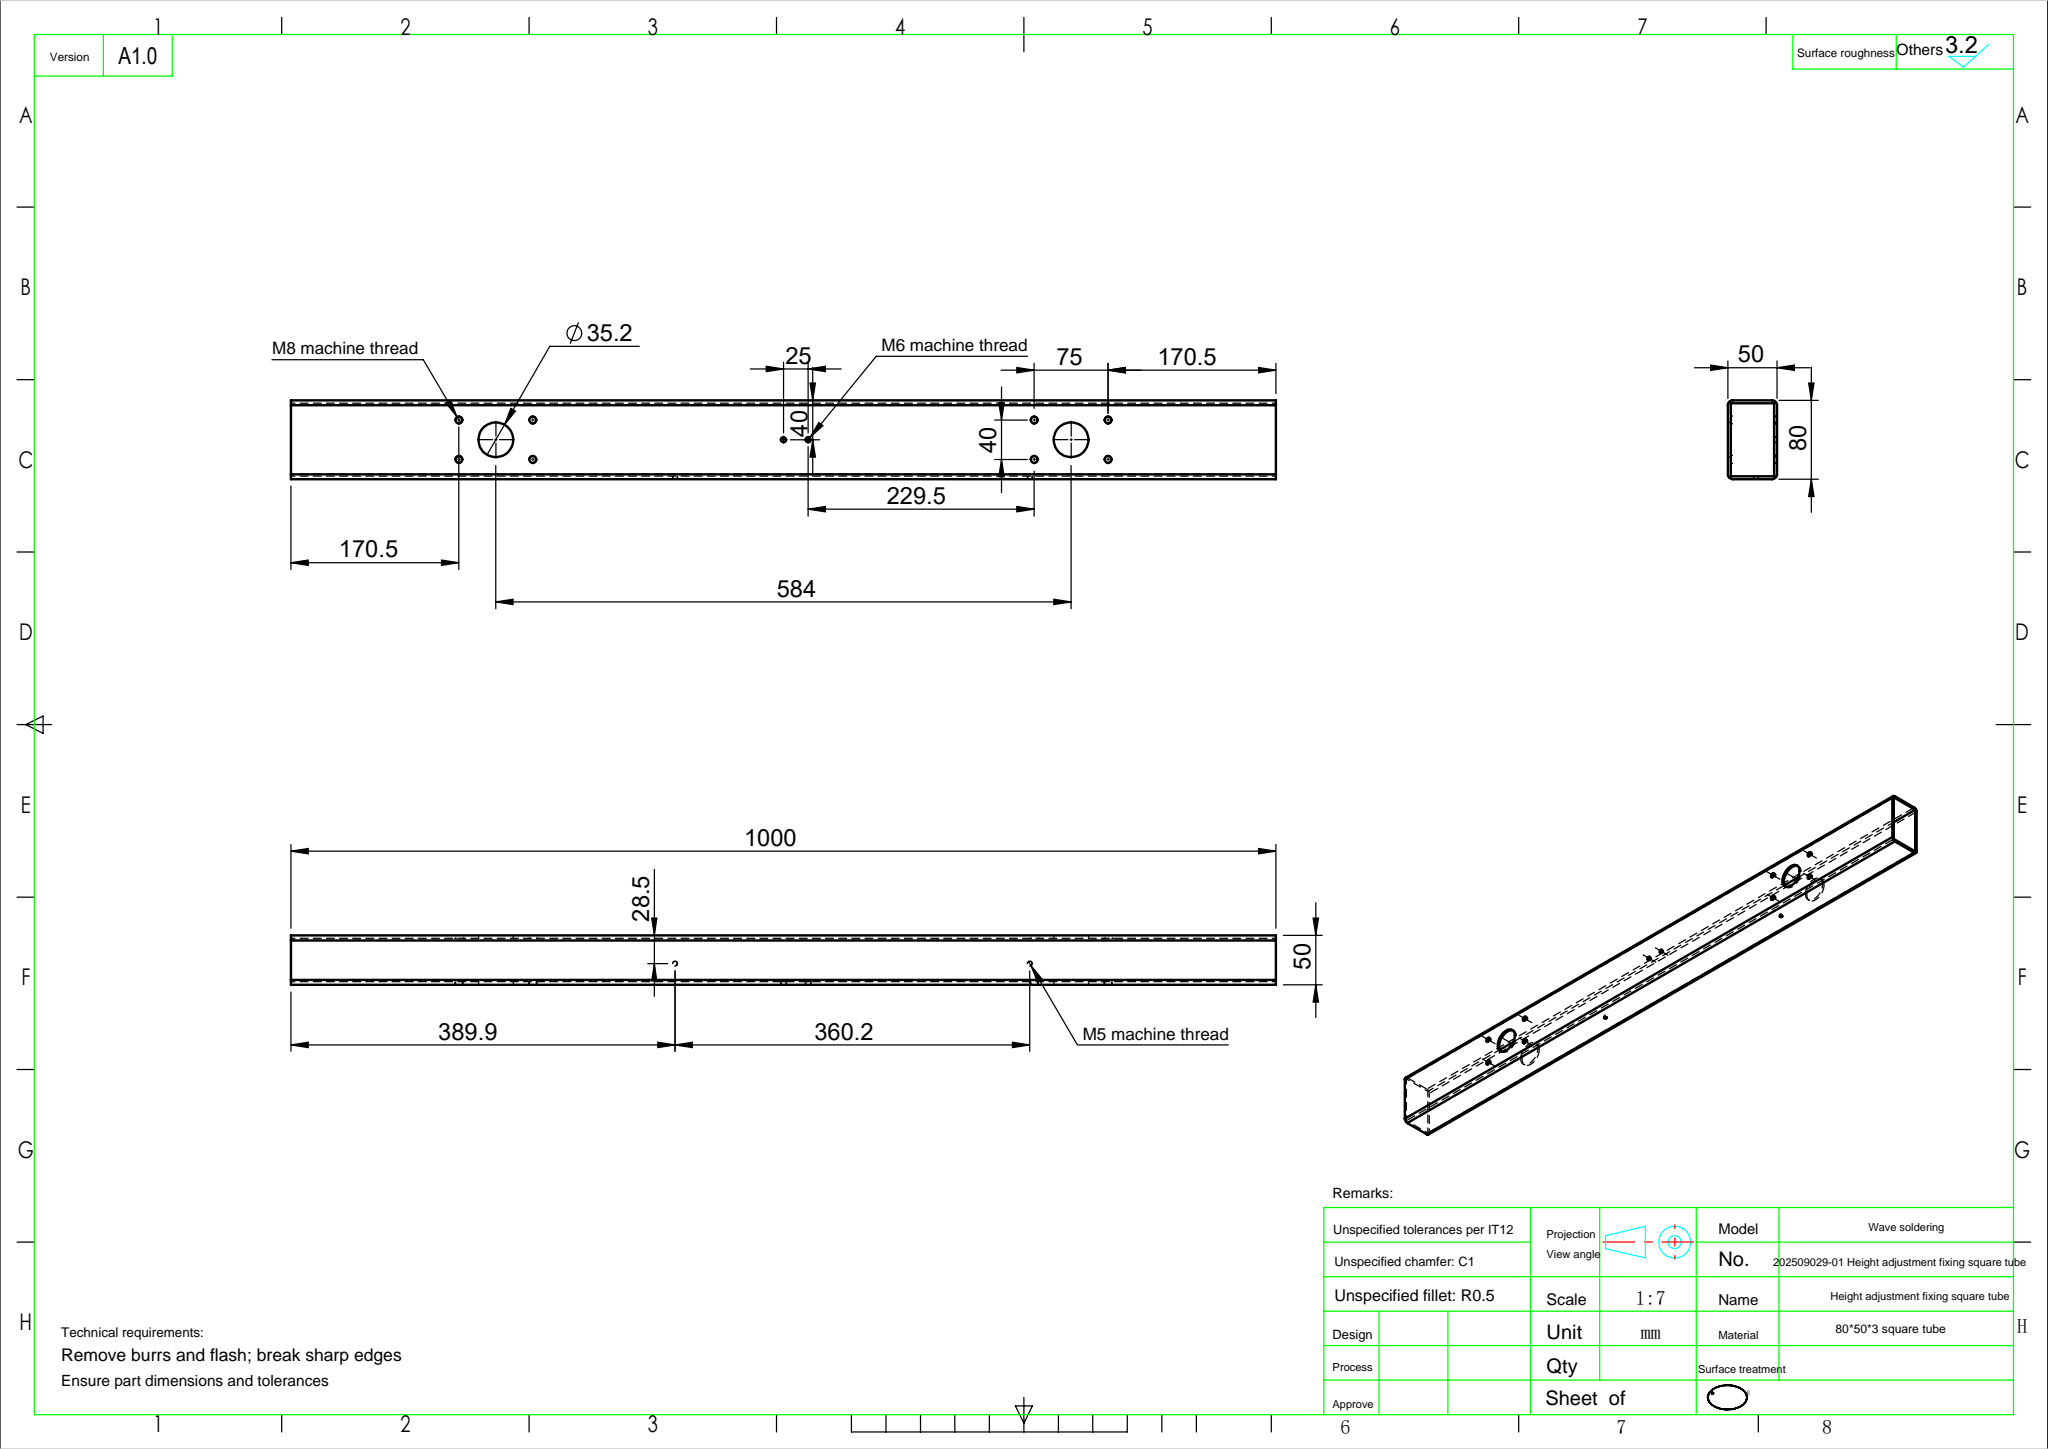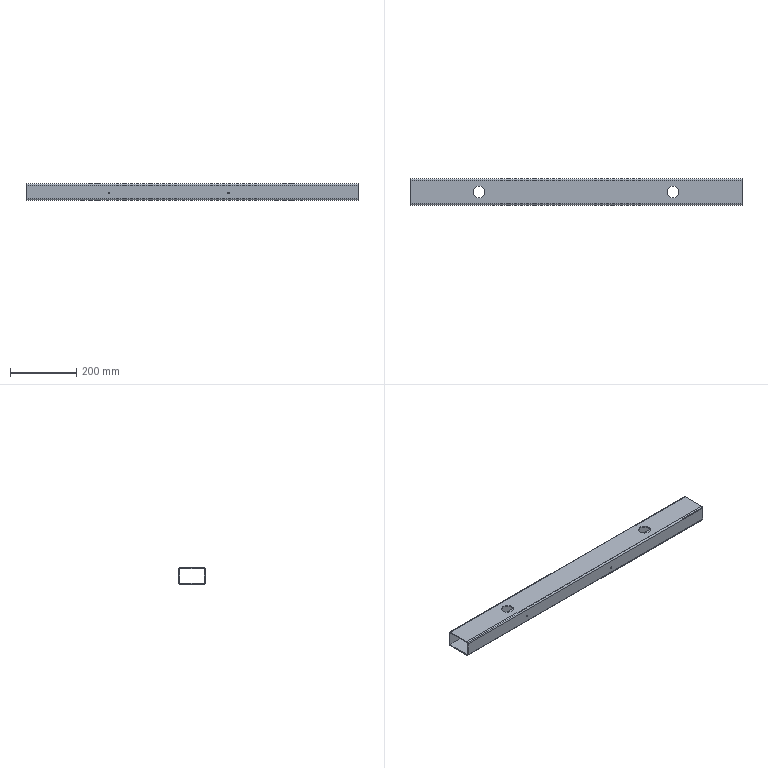Part | SolidWorks | features Cut 2, ICE 2, Extrusion 1, Fillet 1, Shell 1 | 1 solid | 46 faces | box 1000 x 80 x 50 mm | volume 709790 mm3 | cylinder 36 | plane 10 | commonest cylinder face diameters 6.8 x16 35.2 x8 4.2 x4 5 x4 10 x4